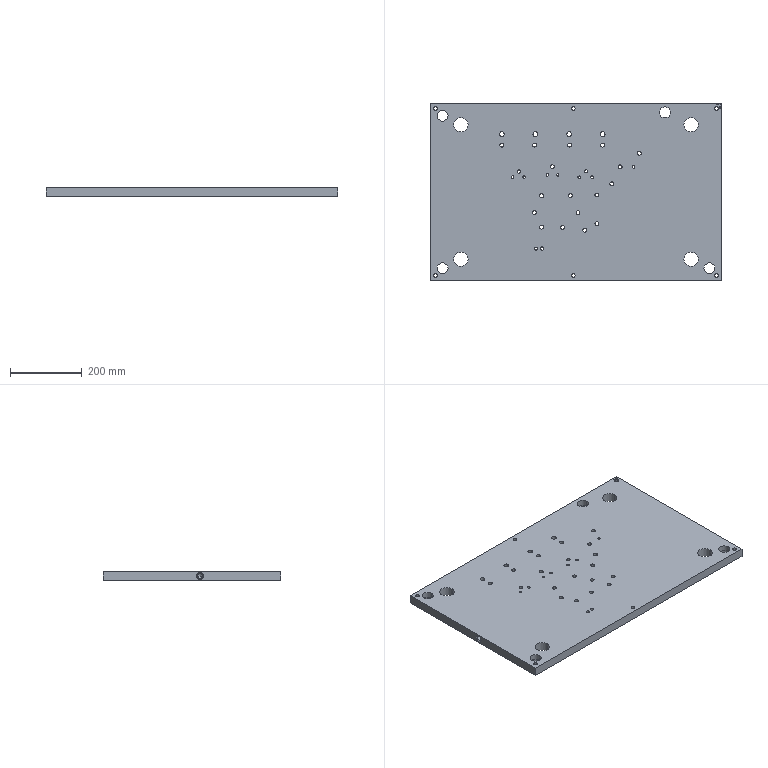Part | Creo | 1 solid | 231 faces | box 815 x 496 x 25 mm | volume 9786673 mm3 | cylinder 140 | plane 77 | cone 14 | commonest cylinder face diameters 11 x41 16 x17 7 x14 10.2 x12 9 x8 13 x8